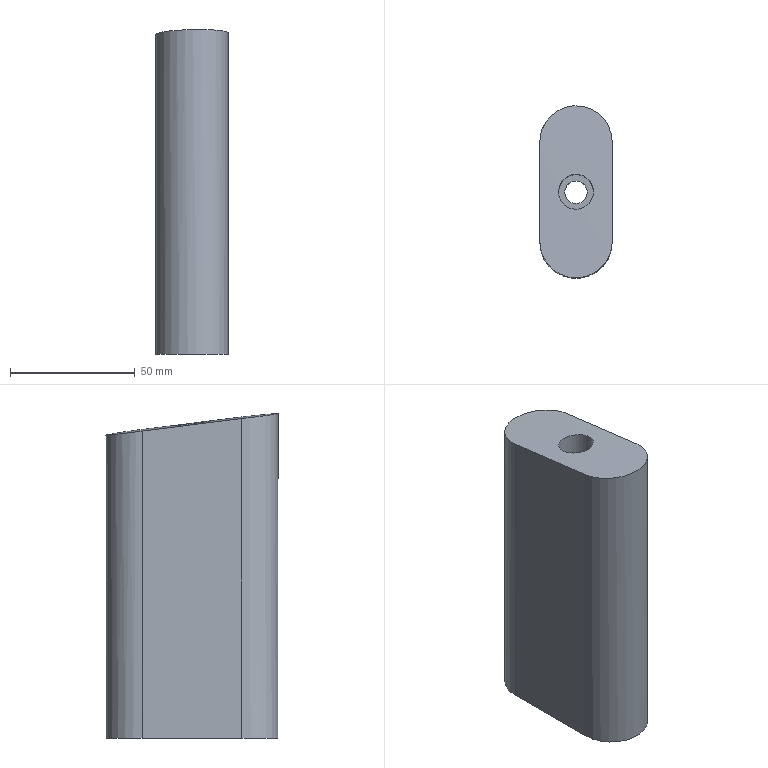Part | NX | features solid 2 | 1 solid | 9 faces | box 29 x 69 x 130.196 mm | volume 211829 mm3 | plane 4 | cylinder 4 | spline 1 | commonest cylinder face diameters 29 x2 9 x1 14 x1
STEP:
#1=CARTESIAN_POINT('',(-261.5,285.,-170.));
#2=VERTEX_POINT('',#1);
#3=CARTESIAN_POINT('',(-261.5,245.,-170.));
#4=VERTEX_POINT('',#3);
#5=CARTESIAN_POINT('',(-261.5,285.,-170.));
#6=DIRECTION('',(0.,-1.,0.));
#7=VECTOR('',#6,1000.);
#8=LINE('',#5,#7);
#9=EDGE_CURVE('',#2,#4,#8,.T.);
#10=ORIENTED_EDGE('',*,*,#9,.F.);
#11=CARTESIAN_POINT('',(-232.5,285.,-170.));
#12=VERTEX_POINT('',#11);
#13=CARTESIAN_POINT('',(-247.,285.,-170.));
#14=DIRECTION('',(0.,0.,1.));
#15=DIRECTION('',(1.,0.,0.));
#16=AXIS2_PLACEMENT_3D('',#13,#14,#15);
#17=CIRCLE('',#16,14.5);
#18=EDGE_CURVE('',#12,#2,#17,.T.);
#19=ORIENTED_EDGE('',*,*,#18,.F.);
#20=CARTESIAN_POINT('',(-232.5,245.,-170.));
#21=VERTEX_POINT('',#20);
#22=CARTESIAN_POINT('',(-232.5,285.,-170.));
#23=DIRECTION('',(0.,-1.,0.));
#24=VECTOR('',#23,1000.);
#25=LINE('',#22,#24);
#26=EDGE_CURVE('',#12,#21,#25,.T.);
#27=ORIENTED_EDGE('',*,*,#26,.T.);
#28=CARTESIAN_POINT('',(-247.,245.,-170.));
#29=DIRECTION('',(0.,0.,1.));
#30=DIRECTION('',(1.,0.,0.));
#31=AXIS2_PLACEMENT_3D('',#28,#29,#30);
#32=CIRCLE('',#31,14.5);
#33=EDGE_CURVE('',#4,#21,#32,.T.);
#34=ORIENTED_EDGE('',*,*,#33,.F.);
#35=EDGE_LOOP('',(#10,#19,#27,#34));
#36=FACE_BOUND('',#35,.T.);
#37=CARTESIAN_POINT('',(-251.5,265.,-170.));
#38=VERTEX_POINT('',#37);
#39=CARTESIAN_POINT('',(-247.,265.,-170.));
#40=DIRECTION('',(0.,0.,-1.));
#41=DIRECTION('',(-1.,0.,0.));
#42=AXIS2_PLACEMENT_3D('',#39,#40,#41);
#43=CIRCLE('',#42,4.5);
#44=EDGE_CURVE('',#38,#38,#43,.F.);
#45=ORIENTED_EDGE('',*,*,#44,.T.);
#46=EDGE_LOOP('',(#45));
#47=FACE_BOUND('',#46,.T.);
#48=CARTESIAN_POINT('',(-247.,285.,-170.));
#49=DIRECTION('',(0.,0.,-1.));
#50=DIRECTION('',(1.,0.,0.));
#51=AXIS2_PLACEMENT_3D('',#48,#49,#50);
#52=PLANE('',#51);
#53=ADVANCED_FACE('',(#36,#47),#52,.T.);
#54=CARTESIAN_POINT('',(-232.5,245.,-41.167));
#55=VERTEX_POINT('',#54);
#56=CARTESIAN_POINT('',(-232.5,245.,-70.));
#57=DIRECTION('',(0.,0.,-1.));
#58=VECTOR('',#57,1000.);
#59=LINE('',#56,#58);
#60=EDGE_CURVE('',#55,#21,#59,.T.);
#61=ORIENTED_EDGE('',*,*,#60,.T.);
#62=ORIENTED_EDGE('',*,*,#26,.F.);
#63=CARTESIAN_POINT('',(-232.5,285.,-46.163));
#64=VERTEX_POINT('',#63);
#65=CARTESIAN_POINT('',(-232.5,285.,-70.));
#66=DIRECTION('',(0.,0.,1.));
#67=VECTOR('',#66,1000.);
#68=LINE('',#65,#67);
#69=EDGE_CURVE('',#64,#12,#68,.F.);
#70=ORIENTED_EDGE('',*,*,#69,.F.);
#71=CARTESIAN_POINT('',(-232.5,285.,-46.163));
#72=CARTESIAN_POINT('',(-232.5,271.682,-44.385));
#73=CARTESIAN_POINT('',(-232.5,258.347,-42.719));
#74=CARTESIAN_POINT('',(-232.5,245.,-41.167));
#75=B_SPLINE_CURVE_WITH_KNOTS('',3,(#71,#72,#73,#74),.UNSPECIFIED.,.F.,.F.,(4,4),(0.06139,0.1017),.UNSPECIFIED.);
#76=EDGE_CURVE('',#64,#55,#75,.T.);
#77=ORIENTED_EDGE('',*,*,#76,.T.);
#78=EDGE_LOOP('',(#61,#62,#70,#77));
#79=FACE_BOUND('',#78,.T.);
#80=CARTESIAN_POINT('',(-232.5,285.,-70.));
#81=DIRECTION('',(1.,0.,0.));
#82=DIRECTION('',(0.,0.,1.));
#83=AXIS2_PLACEMENT_3D('',#80,#81,#82);
#84=PLANE('',#83);
#85=ADVANCED_FACE('',(#79),#84,.T.);
#86=CARTESIAN_POINT('',(-253.959,264.247,-43.954));
#87=VERTEX_POINT('',#86);
#88=CARTESIAN_POINT('',(-251.877,258.967,-43.253));
#89=CARTESIAN_POINT('',(-254.706,264.167,-43.959));
#90=CARTESIAN_POINT('',(-253.056,269.847,-44.637));
#91=CARTESIAN_POINT('',(-247.838,272.72,-44.887));
#92=CARTESIAN_POINT('',(-242.12,271.03,-44.544));
#93=CARTESIAN_POINT('',(-239.297,265.837,-43.825));
#94=CARTESIAN_POINT('',(-240.936,260.162,-43.156));
#95=CARTESIAN_POINT('',(-246.159,257.28,-42.92));
#96=CARTESIAN_POINT('',(-251.877,258.967,-43.253));
#97=CARTESIAN_POINT('',(-254.706,264.167,-43.959));
#98=CARTESIAN_POINT('',(-253.056,269.847,-44.637));
#99=B_SPLINE_CURVE_WITH_KNOTS('',3,(#88,#89,#90,#91,#92,#93,#94,#95,#96,#97,#98),.UNSPECIFIED.,.T.,.F.,(1,1,1,1,1,1,1,1,1,1,1,1,1,1,1),(-0.01648,-0.01098,-0.005492,0.,0.005492,0.01098,0.01648,0.02197,0.02746,0.03295,0.03845,0.04394,0.04943,0.05492,0.06042),.UNSPECIFIED.);
#100=EDGE_CURVE('',#87,#87,#99,.T.);
#101=ORIENTED_EDGE('',*,*,#100,.T.);
#102=EDGE_LOOP('',(#101));
#103=FACE_BOUND('',#102,.T.);
#104=ORIENTED_EDGE('',*,*,#76,.F.);
#105=CARTESIAN_POINT('',(-261.5,285.,-46.814));
#106=VERTEX_POINT('',#105);
#107=CARTESIAN_POINT('',(-232.5,285.,-46.163));
#108=CARTESIAN_POINT('',(-232.5,286.908,-46.418));
#109=CARTESIAN_POINT('',(-233.251,290.659,-46.94));
#110=CARTESIAN_POINT('',(-237.507,297.109,-47.915));
#111=CARTESIAN_POINT('',(-245.05,300.27,-48.523));
#112=CARTESIAN_POINT('',(-252.684,298.75,-48.485));
#113=CARTESIAN_POINT('',(-259.156,294.431,-48.035));
#114=CARTESIAN_POINT('',(-261.5,288.815,-47.324));
#115=CARTESIAN_POINT('',(-261.5,285.,-46.814));
#116=B_SPLINE_CURVE_WITH_KNOTS('',3,(#107,#108,#109,#110,#111,#112,#113,#114,#115),.UNSPECIFIED.,.F.,.F.,(4,1,1,1,1,1,4),(0.,0.005692,0.01138,0.02277,0.02846,0.03415,0.04553),.UNSPECIFIED.);
#117=EDGE_CURVE('',#64,#106,#116,.T.);
#118=ORIENTED_EDGE('',*,*,#117,.T.);
#119=CARTESIAN_POINT('',(-261.5,245.,-41.809));
#120=VERTEX_POINT('',#119);
#121=CARTESIAN_POINT('',(-261.5,285.,-46.814));
#122=CARTESIAN_POINT('',(-261.5,271.682,-45.032));
#123=CARTESIAN_POINT('',(-261.5,258.346,-43.364));
#124=CARTESIAN_POINT('',(-261.5,245.,-41.809));
#125=B_SPLINE_CURVE_WITH_KNOTS('',3,(#121,#122,#123,#124),.UNSPECIFIED.,.F.,.F.,(4,4),(0.1023,0.1426),.UNSPECIFIED.);
#126=EDGE_CURVE('',#106,#120,#125,.T.);
#127=ORIENTED_EDGE('',*,*,#126,.T.);
#128=CARTESIAN_POINT('',(-261.5,245.,-41.809));
#129=CARTESIAN_POINT('',(-261.5,241.233,-41.37));
#130=CARTESIAN_POINT('',(-258.402,233.681,-40.439));
#131=CARTESIAN_POINT('',(-247.029,228.917,-39.659));
#132=CARTESIAN_POINT('',(-235.612,233.652,-39.933));
#133=CARTESIAN_POINT('',(-232.5,241.228,-40.728));
#134=CARTESIAN_POINT('',(-232.5,245.,-41.167));
#135=B_SPLINE_CURVE_WITH_KNOTS('',3,(#128,#129,#130,#131,#132,#133,#134),.UNSPECIFIED.,.F.,.F.,(4,1,1,1,4),(0.06643,0.07779,0.08916,0.1005,0.1119),.UNSPECIFIED.);
#136=EDGE_CURVE('',#120,#55,#135,.T.);
#137=ORIENTED_EDGE('',*,*,#136,.T.);
#138=EDGE_LOOP('',(#104,#118,#127,#137));
#139=FACE_BOUND('',#138,.T.);
#140=CARTESIAN_POINT('',(-261.672,300.045,-48.879));
#141=CARTESIAN_POINT('',(-251.887,300.016,-48.639));
#142=CARTESIAN_POINT('',(-242.103,299.99,-48.415));
#143=CARTESIAN_POINT('',(-232.319,299.965,-48.206));
#144=CARTESIAN_POINT('',(-261.675,276.689,-45.604));
#145=CARTESIAN_POINT('',(-251.891,276.661,-45.366));
#146=CARTESIAN_POINT('',(-242.106,276.634,-45.144));
#147=CARTESIAN_POINT('',(-232.322,276.609,-44.937));
#148=CARTESIAN_POINT('',(-261.679,253.371,-42.686));
#149=CARTESIAN_POINT('',(-251.894,253.343,-42.45));
#150=CARTESIAN_POINT('',(-242.11,253.317,-42.23));
#151=CARTESIAN_POINT('',(-232.325,253.293,-42.025));
#152=CARTESIAN_POINT('',(-261.683,230.092,-40.125));
#153=CARTESIAN_POINT('',(-251.898,230.064,-39.891));
#154=CARTESIAN_POINT('',(-242.113,230.038,-39.672));
#155=CARTESIAN_POINT('',(-232.328,230.014,-39.469));
#156=B_SPLINE_SURFACE_WITH_KNOTS('',3,3,((#140,#141,#142,#143),(#144,#145,#146,#147),(#148,#149,#150,#151),(#152,#153,#154,#155)),.UNSPECIFIED.,.F.,.F.,.F.,(4,4),(4,4),(0.3814,0.4876),(0.4813,0.5171),.UNSPECIFIED.);
#157=ADVANCED_FACE('',(#103,#139),#156,.T.);
#158=CARTESIAN_POINT('',(-261.5,245.,-70.));
#159=DIRECTION('',(0.,0.,-1.));
#160=VECTOR('',#159,1000.);
#161=LINE('',#158,#160);
#162=EDGE_CURVE('',#4,#120,#161,.F.);
#163=ORIENTED_EDGE('',*,*,#162,.T.);
#164=ORIENTED_EDGE('',*,*,#126,.F.);
#165=CARTESIAN_POINT('',(-261.5,285.,-70.));
#166=DIRECTION('',(0.,0.,-1.));
#167=VECTOR('',#166,1000.);
#168=LINE('',#165,#167);
#169=EDGE_CURVE('',#2,#106,#168,.F.);
#170=ORIENTED_EDGE('',*,*,#169,.F.);
#171=ORIENTED_EDGE('',*,*,#9,.T.);
#172=EDGE_LOOP('',(#163,#164,#170,#171));
#173=FACE_BOUND('',#172,.T.);
#174=CARTESIAN_POINT('',(-261.5,285.,-70.));
#175=DIRECTION('',(-1.,0.,0.));
#176=DIRECTION('',(0.,0.,-1.));
#177=AXIS2_PLACEMENT_3D('',#174,#175,#176);
#178=PLANE('',#177);
#179=ADVANCED_FACE('',(#173),#178,.T.);
#180=ORIENTED_EDGE('',*,*,#33,.T.);
#181=ORIENTED_EDGE('',*,*,#60,.F.);
#182=ORIENTED_EDGE('',*,*,#136,.F.);
#183=ORIENTED_EDGE('',*,*,#162,.F.);
#184=EDGE_LOOP('',(#180,#181,#182,#183));
#185=FACE_BOUND('',#184,.T.);
#186=CARTESIAN_POINT('',(-247.,245.,-70.));
#187=DIRECTION('',(0.,0.,-1.));
#188=DIRECTION('',(1.,0.,0.));
#189=AXIS2_PLACEMENT_3D('',#186,#187,#188);
#190=CYLINDRICAL_SURFACE('',#189,14.5);
#191=ADVANCED_FACE('',(#185),#190,.T.);
#192=ORIENTED_EDGE('',*,*,#169,.T.);
#193=ORIENTED_EDGE('',*,*,#117,.F.);
#194=ORIENTED_EDGE('',*,*,#69,.T.);
#195=ORIENTED_EDGE('',*,*,#18,.T.);
#196=EDGE_LOOP('',(#192,#193,#194,#195));
#197=FACE_BOUND('',#196,.T.);
#198=CARTESIAN_POINT('',(-247.,285.,-70.));
#199=DIRECTION('',(0.,0.,-1.));
#200=DIRECTION('',(1.,0.,0.));
#201=AXIS2_PLACEMENT_3D('',#198,#199,#200);
#202=CYLINDRICAL_SURFACE('',#201,14.5);
#203=ADVANCED_FACE('',(#197),#202,.T.);
#204=CARTESIAN_POINT('',(-240.,265.,-150.));
#205=VERTEX_POINT('',#204);
#206=CARTESIAN_POINT('',(-247.,265.,-150.));
#207=DIRECTION('',(0.,0.,1.));
#208=DIRECTION('',(1.,0.,0.));
#209=AXIS2_PLACEMENT_3D('',#206,#207,#208);
#210=CIRCLE('',#209,7.);
#211=EDGE_CURVE('',#205,#205,#210,.T.);
#212=ORIENTED_EDGE('',*,*,#211,.F.);
#213=EDGE_LOOP('',(#212));
#214=FACE_BOUND('',#213,.T.);
#215=ORIENTED_EDGE('',*,*,#100,.F.);
#216=EDGE_LOOP('',(#215));
#217=FACE_BOUND('',#216,.T.);
#218=CARTESIAN_POINT('',(-247.,265.,-150.));
#219=DIRECTION('',(0.,0.,1.));
#220=DIRECTION('',(1.,0.,0.));
#221=AXIS2_PLACEMENT_3D('',#218,#219,#220);
#222=CYLINDRICAL_SURFACE('',#221,7.);
#223=ADVANCED_FACE('',(#214,#217),#222,.F.);
#224=ORIENTED_EDGE('',*,*,#211,.T.);
#225=EDGE_LOOP('',(#224));
#226=FACE_BOUND('',#225,.T.);
#227=CARTESIAN_POINT('',(-242.5,265.,-150.));
#228=VERTEX_POINT('',#227);
#229=CARTESIAN_POINT('',(-247.,265.,-150.));
#230=DIRECTION('',(0.,0.,1.));
#231=DIRECTION('',(1.,0.,0.));
#232=AXIS2_PLACEMENT_3D('',#229,#230,#231);
#233=CIRCLE('',#232,4.5);
#234=EDGE_CURVE('',#228,#228,#233,.F.);
#235=ORIENTED_EDGE('',*,*,#234,.T.);
#236=EDGE_LOOP('',(#235));
#237=FACE_BOUND('',#236,.T.);
#238=CARTESIAN_POINT('',(-247.,265.,-150.));
#239=DIRECTION('',(0.,0.,1.));
#240=DIRECTION('',(1.,0.,0.));
#241=AXIS2_PLACEMENT_3D('',#238,#239,#240);
#242=PLANE('',#241);
#243=ADVANCED_FACE('',(#226,#237),#242,.T.);
#244=ORIENTED_EDGE('',*,*,#44,.F.);
#245=EDGE_LOOP('',(#244));
#246=FACE_BOUND('',#245,.T.);
#247=ORIENTED_EDGE('',*,*,#234,.F.);
#248=EDGE_LOOP('',(#247));
#249=FACE_BOUND('',#248,.T.);
#250=CARTESIAN_POINT('',(-247.,265.,230.));
#251=DIRECTION('',(0.,0.,-1.));
#252=DIRECTION('',(-1.,0.,0.));
#253=AXIS2_PLACEMENT_3D('',#250,#251,#252);
#254=CYLINDRICAL_SURFACE('',#253,4.5);
#255=ADVANCED_FACE('',(#246,#249),#254,.F.);
#256=CLOSED_SHELL('',(#53,#85,#157,#179,#191,#203,#223,#243,#255));
#257=MANIFOLD_SOLID_BREP('',#256);
#258=(LENGTH_UNIT()NAMED_UNIT(*)SI_UNIT(.MILLI.,.METRE.));
#259=UNCERTAINTY_MEASURE_WITH_UNIT(LENGTH_MEASURE(0.0508),#258,'','');
#260=(NAMED_UNIT(*)PLANE_ANGLE_UNIT()SI_UNIT($,.RADIAN.));
#261=(NAMED_UNIT(*)SI_UNIT($,.STERADIAN.)SOLID_ANGLE_UNIT());
#262=(GEOMETRIC_REPRESENTATION_CONTEXT(3)GLOBAL_UNCERTAINTY_ASSIGNED_CONTEXT((#259))GLOBAL_UNIT_ASSIGNED_CONTEXT((#258,#260,#261))REPRESENTATION_CONTEXT('',''));
#263=ADVANCED_BREP_SHAPE_REPRESENTATION('',(#257),#262);